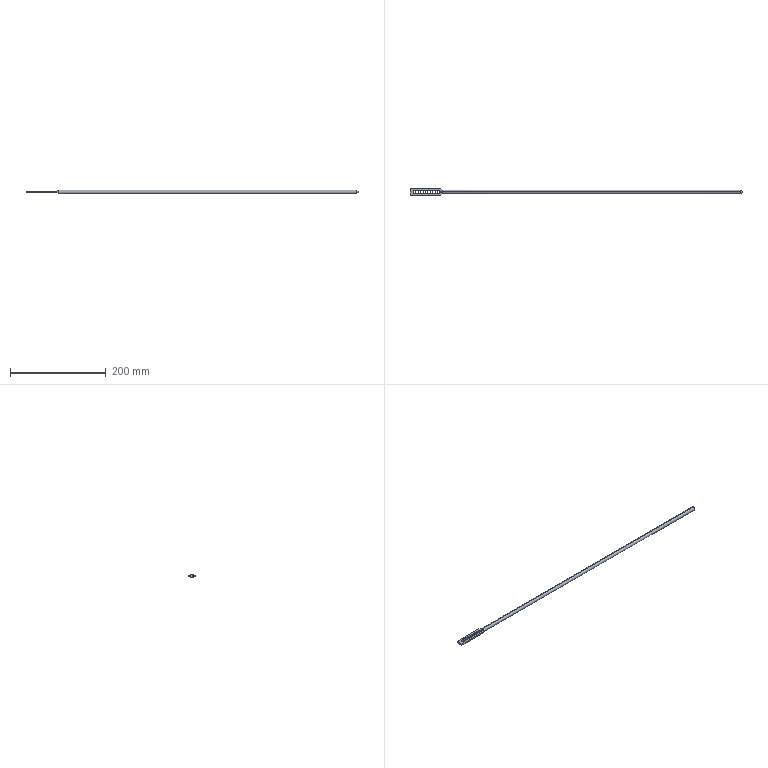Part | SolidWorks | 1 solid | 36 faces | box 695 x 14 x 8 mm | volume 33732 mm3 | cylinder 23 | plane 8 | cone 5 | commonest cylinder face diameters 6.1 x21 8 x2
STEP:
#1=CARTESIAN_POINT('',(67.,3.597,1.75));
#2=VERTEX_POINT('',#1);
#3=CARTESIAN_POINT('',(67.,0.,4.));
#4=VERTEX_POINT('',#3);
#5=CARTESIAN_POINT('',(67.,0.,0.));
#6=DIRECTION('',(1.,0.,0.));
#7=DIRECTION('',(0.,0.,-1.));
#8=AXIS2_PLACEMENT_3D('',#5,#6,#7);
#9=CIRCLE('',#8,4.);
#10=EDGE_CURVE('',#2,#4,#9,.T.);
#11=ORIENTED_EDGE('',*,*,#10,.T.);
#12=CARTESIAN_POINT('',(692.,0.,4.));
#13=VERTEX_POINT('',#12);
#14=CARTESIAN_POINT('',(695.,0.,4.));
#15=DIRECTION('',(1.,0.,0.));
#16=VECTOR('',#15,1000.);
#17=LINE('',#14,#16);
#18=EDGE_CURVE('',#4,#13,#17,.T.);
#19=ORIENTED_EDGE('',*,*,#18,.T.);
#20=CARTESIAN_POINT('',(692.,0.,-4.));
#21=VERTEX_POINT('',#20);
#22=CARTESIAN_POINT('',(692.,0.,0.));
#23=DIRECTION('',(-1.,0.,0.));
#24=DIRECTION('',(0.,0.,-1.));
#25=AXIS2_PLACEMENT_3D('',#22,#23,#24);
#26=CIRCLE('',#25,4.);
#27=EDGE_CURVE('',#13,#21,#26,.T.);
#28=ORIENTED_EDGE('',*,*,#27,.T.);
#29=CARTESIAN_POINT('',(67.,0.,-4.));
#30=VERTEX_POINT('',#29);
#31=CARTESIAN_POINT('',(695.,0.,-4.));
#32=DIRECTION('',(1.,0.,0.));
#33=VECTOR('',#32,1000.);
#34=LINE('',#31,#33);
#35=EDGE_CURVE('',#30,#21,#34,.T.);
#36=ORIENTED_EDGE('',*,*,#35,.F.);
#37=CARTESIAN_POINT('',(67.,3.597,-1.75));
#38=VERTEX_POINT('',#37);
#39=CARTESIAN_POINT('',(67.,0.,0.));
#40=DIRECTION('',(1.,0.,0.));
#41=DIRECTION('',(0.,0.,-1.));
#42=AXIS2_PLACEMENT_3D('',#39,#40,#41);
#43=CIRCLE('',#42,4.);
#44=EDGE_CURVE('',#30,#38,#43,.T.);
#45=ORIENTED_EDGE('',*,*,#44,.T.);
#46=CARTESIAN_POINT('',(67.903,3.597,-1.75));
#47=VERTEX_POINT('',#46);
#48=CARTESIAN_POINT('',(68.,3.597,-1.75));
#49=DIRECTION('',(1.,0.,0.));
#50=VECTOR('',#49,1000.);
#51=LINE('',#48,#50);
#52=EDGE_CURVE('',#38,#47,#51,.T.);
#53=ORIENTED_EDGE('',*,*,#52,.T.);
#54=CARTESIAN_POINT('',(67.903,3.597,1.75));
#55=VERTEX_POINT('',#54);
#56=CARTESIAN_POINT('',(67.903,3.597,-1.75));
#57=CARTESIAN_POINT('',(67.356,4.144,-0.6253));
#58=CARTESIAN_POINT('',(67.356,4.144,0.6253));
#59=CARTESIAN_POINT('',(67.903,3.597,1.75));
#60=(BOUNDED_CURVE()B_SPLINE_CURVE(3,(#56,#57,#58,#59),.UNSPECIFIED.,.F.,.F.)B_SPLINE_CURVE_WITH_KNOTS((4,4),(2.689,3.594),.UNSPECIFIED.)CURVE()GEOMETRIC_REPRESENTATION_ITEM()RATIONAL_B_SPLINE_CURVE((1.,0.9328,0.9328,1.))REPRESENTATION_ITEM(''));
#61=EDGE_CURVE('',#47,#55,#60,.T.);
#62=ORIENTED_EDGE('',*,*,#61,.T.);
#63=CARTESIAN_POINT('',(0.,3.597,1.75));
#64=DIRECTION('',(-1.,0.,0.));
#65=VECTOR('',#64,1000.);
#66=LINE('',#63,#65);
#67=EDGE_CURVE('',#55,#2,#66,.T.);
#68=ORIENTED_EDGE('',*,*,#67,.T.);
#69=EDGE_LOOP('',(#11,#19,#28,#36,#45,#53,#62,#68));
#70=FACE_OUTER_BOUND('',#69,.T.);
#71=CARTESIAN_POINT('',(695.,0.,0.));
#72=DIRECTION('',(1.,0.,0.));
#73=DIRECTION('',(0.,0.,-1.));
#74=AXIS2_PLACEMENT_3D('',#71,#72,#73);
#75=CYLINDRICAL_SURFACE('',#74,4.);
#76=ADVANCED_FACE('',(#70),#75,.T.);
#77=CARTESIAN_POINT('',(67.,-3.597,-1.75));
#78=VERTEX_POINT('',#77);
#79=CARTESIAN_POINT('',(65.678,0.,-1.75));
#80=VERTEX_POINT('',#79);
#81=CARTESIAN_POINT('',(67.,-3.597,-1.75));
#82=CARTESIAN_POINT('',(66.849,-3.312,-1.75));
#83=CARTESIAN_POINT('',(66.701,-3.025,-1.75));
#84=CARTESIAN_POINT('',(66.416,-2.448,-1.75));
#85=CARTESIAN_POINT('',(66.277,-2.157,-1.75));
#86=CARTESIAN_POINT('',(66.024,-1.564,-1.75));
#87=CARTESIAN_POINT('',(65.907,-1.262,-1.75));
#88=CARTESIAN_POINT('',(65.777,-0.7984,-1.75));
#89=CARTESIAN_POINT('',(65.741,-0.642,-1.75));
#90=CARTESIAN_POINT('',(65.692,-0.3236,-1.75));
#91=CARTESIAN_POINT('',(65.678,-0.1604,-1.75));
#92=CARTESIAN_POINT('',(65.678,0.,-1.75));
#93=B_SPLINE_CURVE_WITH_KNOTS('',3,(#81,#82,#83,#84,#85,#86,#87,#88,#89,#90,#91,#92),.UNSPECIFIED.,.F.,.F.,(4,2,2,2,2,4),(0.,0.0009664,0.001933,0.002899,0.003382,0.003866),.UNSPECIFIED.);
#94=EDGE_CURVE('',#78,#80,#93,.T.);
#95=ORIENTED_EDGE('',*,*,#94,.T.);
#96=CARTESIAN_POINT('',(67.,0.,-4.));
#97=DIRECTION('',(0.5065,0.,-0.8622));
#98=VECTOR('',#97,1000.);
#99=LINE('',#96,#98);
#100=EDGE_CURVE('',#80,#30,#99,.T.);
#101=ORIENTED_EDGE('',*,*,#100,.T.);
#102=CARTESIAN_POINT('',(67.,0.,0.));
#103=DIRECTION('',(1.,0.,0.));
#104=DIRECTION('',(0.,0.,-1.));
#105=AXIS2_PLACEMENT_3D('',#102,#103,#104);
#106=CIRCLE('',#105,4.);
#107=EDGE_CURVE('',#78,#30,#106,.T.);
#108=ORIENTED_EDGE('',*,*,#107,.F.);
#109=EDGE_LOOP('',(#95,#101,#108));
#110=FACE_OUTER_BOUND('',#109,.T.);
#111=CARTESIAN_POINT('',(67.,0.,0.));
#112=DIRECTION('',(1.,0.,0.));
#113=DIRECTION('',(0.,0.,-1.));
#114=AXIS2_PLACEMENT_3D('',#111,#112,#113);
#115=CONICAL_SURFACE('',#114,4.,1.04);
#116=ADVANCED_FACE('',(#110),#115,.T.);
#117=CARTESIAN_POINT('',(695.,0.,1.5));
#118=VERTEX_POINT('',#117);
#119=CARTESIAN_POINT('',(695.,0.,-1.5));
#120=VERTEX_POINT('',#119);
#121=CARTESIAN_POINT('',(695.,0.,0.));
#122=DIRECTION('',(-1.,0.,0.));
#123=DIRECTION('',(0.,0.,1.));
#124=AXIS2_PLACEMENT_3D('',#121,#122,#123);
#125=CIRCLE('',#124,1.5);
#126=EDGE_CURVE('',#118,#120,#125,.T.);
#127=ORIENTED_EDGE('',*,*,#126,.T.);
#128=CARTESIAN_POINT('',(692.,0.,-4.));
#129=DIRECTION('',(-0.7682,0.,-0.6402));
#130=VECTOR('',#129,1000.);
#131=LINE('',#128,#130);
#132=EDGE_CURVE('',#120,#21,#131,.T.);
#133=ORIENTED_EDGE('',*,*,#132,.T.);
#134=ORIENTED_EDGE('',*,*,#27,.F.);
#135=CARTESIAN_POINT('',(692.,0.,4.));
#136=DIRECTION('',(-0.7682,0.,0.6402));
#137=VECTOR('',#136,1000.);
#138=LINE('',#135,#137);
#139=EDGE_CURVE('',#118,#13,#138,.T.);
#140=ORIENTED_EDGE('',*,*,#139,.F.);
#141=EDGE_LOOP('',(#127,#133,#134,#140));
#142=FACE_OUTER_BOUND('',#141,.T.);
#143=CARTESIAN_POINT('',(692.,0.,0.));
#144=DIRECTION('',(-1.,0.,0.));
#145=DIRECTION('',(0.,0.,1.));
#146=AXIS2_PLACEMENT_3D('',#143,#144,#145);
#147=CONICAL_SURFACE('',#146,4.,0.6947);
#148=ADVANCED_FACE('',(#142),#147,.T.);
#149=CARTESIAN_POINT('',(12.5,1.747,1.75));
#150=VERTEX_POINT('',#149);
#151=CARTESIAN_POINT('',(6.95,0.,1.75));
#152=VERTEX_POINT('',#151);
#153=CARTESIAN_POINT('',(10.,0.,1.75));
#154=DIRECTION('',(0.,0.,1.));
#155=DIRECTION('',(-1.,0.,0.));
#156=AXIS2_PLACEMENT_3D('',#153,#154,#155);
#157=CIRCLE('',#156,3.05);
#158=EDGE_CURVE('',#150,#152,#157,.T.);
#159=ORIENTED_EDGE('',*,*,#158,.T.);
#160=CARTESIAN_POINT('',(6.95,0.,-1.75));
#161=VERTEX_POINT('',#160);
#162=CARTESIAN_POINT('',(6.95,0.,7.));
#163=DIRECTION('',(0.,0.,-1.));
#164=VECTOR('',#163,1000.);
#165=LINE('',#162,#164);
#166=EDGE_CURVE('',#152,#161,#165,.T.);
#167=ORIENTED_EDGE('',*,*,#166,.T.);
#168=CARTESIAN_POINT('',(12.5,1.747,-1.75));
#169=VERTEX_POINT('',#168);
#170=CARTESIAN_POINT('',(10.,0.,-1.75));
#171=DIRECTION('',(0.,0.,-1.));
#172=DIRECTION('',(-1.,0.,0.));
#173=AXIS2_PLACEMENT_3D('',#170,#171,#172);
#174=CIRCLE('',#173,3.05);
#175=EDGE_CURVE('',#161,#169,#174,.T.);
#176=ORIENTED_EDGE('',*,*,#175,.T.);
#177=CARTESIAN_POINT('',(12.5,1.747,7.));
#178=DIRECTION('',(0.,0.,1.));
#179=VECTOR('',#178,1000.);
#180=LINE('',#177,#179);
#181=EDGE_CURVE('',#169,#150,#180,.T.);
#182=ORIENTED_EDGE('',*,*,#181,.T.);
#183=EDGE_LOOP('',(#159,#167,#176,#182));
#184=FACE_OUTER_BOUND('',#183,.T.);
#185=CARTESIAN_POINT('',(10.,0.,7.));
#186=DIRECTION('',(0.,0.,-1.));
#187=DIRECTION('',(-1.,0.,0.));
#188=AXIS2_PLACEMENT_3D('',#185,#186,#187);
#189=CYLINDRICAL_SURFACE('',#188,3.05);
#190=ADVANCED_FACE('',(#184),#189,.F.);
#191=ORIENTED_EDGE('',*,*,#18,.F.);
#192=CARTESIAN_POINT('',(67.,-3.597,1.75));
#193=VERTEX_POINT('',#192);
#194=CARTESIAN_POINT('',(67.,0.,0.));
#195=DIRECTION('',(1.,0.,0.));
#196=DIRECTION('',(0.,0.,-1.));
#197=AXIS2_PLACEMENT_3D('',#194,#195,#196);
#198=CIRCLE('',#197,4.);
#199=EDGE_CURVE('',#4,#193,#198,.T.);
#200=ORIENTED_EDGE('',*,*,#199,.T.);
#201=CARTESIAN_POINT('',(67.903,-3.597,1.75));
#202=VERTEX_POINT('',#201);
#203=CARTESIAN_POINT('',(0.,-3.597,1.75));
#204=DIRECTION('',(1.,0.,0.));
#205=VECTOR('',#204,1000.);
#206=LINE('',#203,#205);
#207=EDGE_CURVE('',#193,#202,#206,.T.);
#208=ORIENTED_EDGE('',*,*,#207,.T.);
#209=CARTESIAN_POINT('',(67.903,-3.597,-1.75));
#210=VERTEX_POINT('',#209);
#211=CARTESIAN_POINT('',(67.903,-3.597,1.75));
#212=CARTESIAN_POINT('',(67.356,-4.144,0.6253));
#213=CARTESIAN_POINT('',(67.356,-4.144,-0.6253));
#214=CARTESIAN_POINT('',(67.903,-3.597,-1.75));
#215=(BOUNDED_CURVE()B_SPLINE_CURVE(3,(#211,#212,#213,#214),.UNSPECIFIED.,.F.,.F.)B_SPLINE_CURVE_WITH_KNOTS((4,4),(2.689,3.594),.UNSPECIFIED.)CURVE()GEOMETRIC_REPRESENTATION_ITEM()RATIONAL_B_SPLINE_CURVE((1.,0.9328,0.9328,1.))REPRESENTATION_ITEM(''));
#216=EDGE_CURVE('',#202,#210,#215,.T.);
#217=ORIENTED_EDGE('',*,*,#216,.T.);
#218=CARTESIAN_POINT('',(68.,-3.597,-1.75));
#219=DIRECTION('',(-1.,0.,0.));
#220=VECTOR('',#219,1000.);
#221=LINE('',#218,#220);
#222=EDGE_CURVE('',#210,#78,#221,.T.);
#223=ORIENTED_EDGE('',*,*,#222,.T.);
#224=ORIENTED_EDGE('',*,*,#107,.T.);
#225=ORIENTED_EDGE('',*,*,#35,.T.);
#226=CARTESIAN_POINT('',(692.,0.,0.));
#227=DIRECTION('',(-1.,0.,0.));
#228=DIRECTION('',(0.,0.,-1.));
#229=AXIS2_PLACEMENT_3D('',#226,#227,#228);
#230=CIRCLE('',#229,4.);
#231=EDGE_CURVE('',#21,#13,#230,.T.);
#232=ORIENTED_EDGE('',*,*,#231,.T.);
#233=EDGE_LOOP('',(#191,#200,#208,#217,#223,#224,#225,#232));
#234=FACE_OUTER_BOUND('',#233,.T.);
#235=CARTESIAN_POINT('',(695.,0.,0.));
#236=DIRECTION('',(1.,0.,0.));
#237=DIRECTION('',(0.,0.,-1.));
#238=AXIS2_PLACEMENT_3D('',#235,#236,#237);
#239=CYLINDRICAL_SURFACE('',#238,4.);
#240=ADVANCED_FACE('',(#234),#239,.T.);
#241=ORIENTED_EDGE('',*,*,#216,.F.);
#242=CARTESIAN_POINT('',(64.5,-7.,1.75));
#243=VERTEX_POINT('',#242);
#244=CARTESIAN_POINT('',(68.,-3.5,1.75));
#245=DIRECTION('',(0.7071,0.7071,0.));
#246=VECTOR('',#245,1000.);
#247=LINE('',#244,#246);
#248=EDGE_CURVE('',#243,#202,#247,.T.);
#249=ORIENTED_EDGE('',*,*,#248,.F.);
#250=CARTESIAN_POINT('',(64.5,-7.,-1.75));
#251=VERTEX_POINT('',#250);
#252=CARTESIAN_POINT('',(64.5,-7.,1.75));
#253=DIRECTION('',(0.,0.,1.));
#254=VECTOR('',#253,1000.);
#255=LINE('',#252,#254);
#256=EDGE_CURVE('',#251,#243,#255,.T.);
#257=ORIENTED_EDGE('',*,*,#256,.F.);
#258=CARTESIAN_POINT('',(68.,-3.5,-1.75));
#259=DIRECTION('',(-0.7071,-0.7071,0.));
#260=VECTOR('',#259,1000.);
#261=LINE('',#258,#260);
#262=EDGE_CURVE('',#210,#251,#261,.T.);
#263=ORIENTED_EDGE('',*,*,#262,.F.);
#264=EDGE_LOOP('',(#241,#249,#257,#263));
#265=FACE_OUTER_BOUND('',#264,.T.);
#266=CARTESIAN_POINT('',(68.,-3.5,1.75));
#267=DIRECTION('',(-0.7071,0.7071,0.));
#268=DIRECTION('',(-0.7071,-0.7071,0.));
#269=AXIS2_PLACEMENT_3D('',#266,#267,#268);
#270=PLANE('',#269);
#271=ADVANCED_FACE('',(#265),#270,.F.);
#272=ORIENTED_EDGE('',*,*,#10,.F.);
#273=CARTESIAN_POINT('',(67.,3.597,1.75));
#274=CARTESIAN_POINT('',(66.849,3.311,1.75));
#275=CARTESIAN_POINT('',(66.701,3.024,1.75));
#276=CARTESIAN_POINT('',(66.414,2.445,1.75));
#277=CARTESIAN_POINT('',(66.276,2.153,1.75));
#278=CARTESIAN_POINT('',(66.022,1.559,1.75));
#279=CARTESIAN_POINT('',(65.905,1.255,1.75));
#280=CARTESIAN_POINT('',(65.775,0.7905,1.75));
#281=CARTESIAN_POINT('',(65.74,0.6336,1.75));
#282=CARTESIAN_POINT('',(65.691,0.3142,1.75));
#283=CARTESIAN_POINT('',(65.678,0.1505,1.75));
#284=CARTESIAN_POINT('',(65.679,-0.3318,1.75));
#285=CARTESIAN_POINT('',(65.734,-0.6464,1.75));
#286=CARTESIAN_POINT('',(65.909,-1.267,1.75));
#287=CARTESIAN_POINT('',(66.026,-1.569,1.75));
#288=CARTESIAN_POINT('',(66.279,-2.16,1.75));
#289=CARTESIAN_POINT('',(66.417,-2.45,1.75));
#290=CARTESIAN_POINT('',(66.702,-3.027,1.75));
#291=CARTESIAN_POINT('',(66.85,-3.312,1.75));
#292=CARTESIAN_POINT('',(67.,-3.597,1.75));
#293=B_SPLINE_CURVE_WITH_KNOTS('',3,(#273,#274,#275,#276,#277,#278,#279,#280,#281,#282,#283,#284,#285,#286,#287,#288,#289,#290,#291,#292),.UNSPECIFIED.,.F.,.F.,(4,2,2,2,2,2,2,2,2,4),(0.,0.000969,0.001938,0.002907,0.003392,0.003876,0.004845,0.005814,0.006783,0.007752),.UNSPECIFIED.);
#294=EDGE_CURVE('',#2,#193,#293,.T.);
#295=ORIENTED_EDGE('',*,*,#294,.T.);
#296=ORIENTED_EDGE('',*,*,#199,.F.);
#297=EDGE_LOOP('',(#272,#295,#296));
#298=FACE_OUTER_BOUND('',#297,.T.);
#299=CARTESIAN_POINT('',(67.,0.,0.));
#300=DIRECTION('',(1.,0.,0.));
#301=DIRECTION('',(0.,0.,-1.));
#302=AXIS2_PLACEMENT_3D('',#299,#300,#301);
#303=CONICAL_SURFACE('',#302,4.,1.04);
#304=ADVANCED_FACE('',(#298),#303,.T.);
#305=CARTESIAN_POINT('',(64.5,7.,-1.75));
#306=VERTEX_POINT('',#305);
#307=CARTESIAN_POINT('',(64.5,7.,-1.75));
#308=DIRECTION('',(-0.7071,0.7071,0.));
#309=VECTOR('',#308,1000.);
#310=LINE('',#307,#309);
#311=EDGE_CURVE('',#47,#306,#310,.T.);
#312=ORIENTED_EDGE('',*,*,#311,.T.);
#313=CARTESIAN_POINT('',(64.5,7.,1.75));
#314=VERTEX_POINT('',#313);
#315=CARTESIAN_POINT('',(64.5,7.,0.));
#316=DIRECTION('',(0.,0.,1.));
#317=VECTOR('',#316,1000.);
#318=LINE('',#315,#317);
#319=EDGE_CURVE('',#306,#314,#318,.T.);
#320=ORIENTED_EDGE('',*,*,#319,.T.);
#321=CARTESIAN_POINT('',(64.5,7.,1.75));
#322=DIRECTION('',(0.7071,-0.7071,0.));
#323=VECTOR('',#322,1000.);
#324=LINE('',#321,#323);
#325=EDGE_CURVE('',#314,#55,#324,.T.);
#326=ORIENTED_EDGE('',*,*,#325,.T.);
#327=ORIENTED_EDGE('',*,*,#61,.F.);
#328=EDGE_LOOP('',(#312,#320,#326,#327));
#329=FACE_OUTER_BOUND('',#328,.T.);
#330=CARTESIAN_POINT('',(64.5,7.,0.));
#331=DIRECTION('',(0.7071,0.7071,0.));
#332=DIRECTION('',(-0.7071,0.7071,0.));
#333=AXIS2_PLACEMENT_3D('',#330,#331,#332);
#334=PLANE('',#333);
#335=ADVANCED_FACE('',(#329),#334,.T.);
#336=ORIENTED_EDGE('',*,*,#100,.F.);
#337=CARTESIAN_POINT('',(65.678,0.,-1.75));
#338=CARTESIAN_POINT('',(65.678,0.3225,-1.75));
#339=CARTESIAN_POINT('',(65.732,0.6381,-1.75));
#340=CARTESIAN_POINT('',(65.907,1.261,-1.75));
#341=CARTESIAN_POINT('',(66.024,1.564,-1.75));
#342=CARTESIAN_POINT('',(66.277,2.156,-1.75));
#343=CARTESIAN_POINT('',(66.415,2.447,-1.75));
#344=CARTESIAN_POINT('',(66.701,3.025,-1.75));
#345=CARTESIAN_POINT('',(66.849,3.312,-1.75));
#346=CARTESIAN_POINT('',(67.,3.597,-1.75));
#347=B_SPLINE_CURVE_WITH_KNOTS('',3,(#337,#338,#339,#340,#341,#342,#343,#344,#345,#346),.UNSPECIFIED.,.F.,.F.,(4,2,2,2,4),(0.003866,0.004837,0.005809,0.00678,0.007752),.UNSPECIFIED.);
#348=EDGE_CURVE('',#80,#38,#347,.T.);
#349=ORIENTED_EDGE('',*,*,#348,.T.);
#350=ORIENTED_EDGE('',*,*,#44,.F.);
#351=EDGE_LOOP('',(#336,#349,#350));
#352=FACE_OUTER_BOUND('',#351,.T.);
#353=CARTESIAN_POINT('',(67.,0.,0.));
#354=DIRECTION('',(1.,0.,0.));
#355=DIRECTION('',(0.,0.,-1.));
#356=AXIS2_PLACEMENT_3D('',#353,#354,#355);
#357=CONICAL_SURFACE('',#356,4.,1.04);
#358=ADVANCED_FACE('',(#352),#357,.T.);
#359=ORIENTED_EDGE('',*,*,#132,.F.);
#360=CARTESIAN_POINT('',(695.,0.,0.));
#361=DIRECTION('',(-1.,0.,0.));
#362=DIRECTION('',(0.,0.,1.));
#363=AXIS2_PLACEMENT_3D('',#360,#361,#362);
#364=CIRCLE('',#363,1.5);
#365=EDGE_CURVE('',#120,#118,#364,.T.);
#366=ORIENTED_EDGE('',*,*,#365,.T.);
#367=ORIENTED_EDGE('',*,*,#139,.T.);
#368=ORIENTED_EDGE('',*,*,#231,.F.);
#369=EDGE_LOOP('',(#359,#366,#367,#368));
#370=FACE_OUTER_BOUND('',#369,.T.);
#371=CARTESIAN_POINT('',(692.,0.,0.));
#372=DIRECTION('',(-1.,0.,0.));
#373=DIRECTION('',(0.,0.,1.));
#374=AXIS2_PLACEMENT_3D('',#371,#372,#373);
#375=CONICAL_SURFACE('',#374,4.,0.6947);
#376=ADVANCED_FACE('',(#370),#375,.T.);
#377=ORIENTED_EDGE('',*,*,#262,.T.);
#378=CARTESIAN_POINT('',(0.,-7.,-1.75));
#379=VERTEX_POINT('',#378);
#380=CARTESIAN_POINT('',(68.,-7.,-1.75));
#381=DIRECTION('',(1.,0.,0.));
#382=VECTOR('',#381,1000.);
#383=LINE('',#380,#382);
#384=EDGE_CURVE('',#379,#251,#383,.T.);
#385=ORIENTED_EDGE('',*,*,#384,.F.);
#386=CARTESIAN_POINT('',(0.,7.,-1.75));
#387=VERTEX_POINT('',#386);
#388=CARTESIAN_POINT('',(0.,7.,-1.75));
#389=DIRECTION('',(0.,-1.,0.));
#390=VECTOR('',#389,1000.);
#391=LINE('',#388,#390);
#392=EDGE_CURVE('',#387,#379,#391,.T.);
#393=ORIENTED_EDGE('',*,*,#392,.F.);
#394=CARTESIAN_POINT('',(68.,7.,-1.75));
#395=DIRECTION('',(-1.,0.,0.));
#396=VECTOR('',#395,1000.);
#397=LINE('',#394,#396);
#398=EDGE_CURVE('',#306,#387,#397,.T.);
#399=ORIENTED_EDGE('',*,*,#398,.F.);
#400=ORIENTED_EDGE('',*,*,#311,.F.);
#401=ORIENTED_EDGE('',*,*,#52,.F.);
#402=ORIENTED_EDGE('',*,*,#348,.F.);
#403=ORIENTED_EDGE('',*,*,#94,.F.);
#404=ORIENTED_EDGE('',*,*,#222,.F.);
#405=EDGE_LOOP('',(#377,#385,#393,#399,#400,#401,#402,#403,#404));
#406=FACE_OUTER_BOUND('',#405,.T.);
#407=CARTESIAN_POINT('',(22.5,-1.747,-1.75));
#408=VERTEX_POINT('',#407);
#409=CARTESIAN_POINT('',(17.5,-1.747,-1.75));
#410=VERTEX_POINT('',#409);
#411=CARTESIAN_POINT('',(20.,0.,-1.75));
#412=DIRECTION('',(0.,0.,-1.));
#413=DIRECTION('',(-1.,0.,0.));
#414=AXIS2_PLACEMENT_3D('',#411,#412,#413);
#415=CIRCLE('',#414,3.05);
#416=EDGE_CURVE('',#408,#410,#415,.T.);
#417=ORIENTED_EDGE('',*,*,#416,.F.);
#418=CARTESIAN_POINT('',(27.5,-1.747,-1.75));
#419=VERTEX_POINT('',#418);
#420=CARTESIAN_POINT('',(25.,0.,-1.75));
#421=DIRECTION('',(0.,0.,-1.));
#422=DIRECTION('',(-1.,0.,0.));
#423=AXIS2_PLACEMENT_3D('',#420,#421,#422);
#424=CIRCLE('',#423,3.05);
#425=EDGE_CURVE('',#419,#408,#424,.T.);
#426=ORIENTED_EDGE('',*,*,#425,.F.);
#427=CARTESIAN_POINT('',(32.5,-1.747,-1.75));
#428=VERTEX_POINT('',#427);
#429=CARTESIAN_POINT('',(30.,0.,-1.75));
#430=DIRECTION('',(0.,0.,-1.));
#431=DIRECTION('',(-1.,0.,0.));
#432=AXIS2_PLACEMENT_3D('',#429,#430,#431);
#433=CIRCLE('',#432,3.05);
#434=EDGE_CURVE('',#428,#419,#433,.T.);
#435=ORIENTED_EDGE('',*,*,#434,.F.);
#436=CARTESIAN_POINT('',(37.5,-1.747,-1.75));
#437=VERTEX_POINT('',#436);
#438=CARTESIAN_POINT('',(35.,0.,-1.75));
#439=DIRECTION('',(0.,0.,-1.));
#440=DIRECTION('',(-1.,0.,0.));
#441=AXIS2_PLACEMENT_3D('',#438,#439,#440);
#442=CIRCLE('',#441,3.05);
#443=EDGE_CURVE('',#437,#428,#442,.T.);
#444=ORIENTED_EDGE('',*,*,#443,.F.);
#445=CARTESIAN_POINT('',(42.5,-1.747,-1.75));
#446=VERTEX_POINT('',#445);
#447=CARTESIAN_POINT('',(40.,0.,-1.75));
#448=DIRECTION('',(0.,0.,-1.));
#449=DIRECTION('',(-1.,0.,0.));
#450=AXIS2_PLACEMENT_3D('',#447,#448,#449);
#451=CIRCLE('',#450,3.05);
#452=EDGE_CURVE('',#446,#437,#451,.T.);
#453=ORIENTED_EDGE('',*,*,#452,.F.);
#454=CARTESIAN_POINT('',(47.5,-1.747,-1.75));
#455=VERTEX_POINT('',#454);
#456=CARTESIAN_POINT('',(45.,0.,-1.75));
#457=DIRECTION('',(0.,0.,-1.));
#458=DIRECTION('',(-1.,0.,0.));
#459=AXIS2_PLACEMENT_3D('',#456,#457,#458);
#460=CIRCLE('',#459,3.05);
#461=EDGE_CURVE('',#455,#446,#460,.T.);
#462=ORIENTED_EDGE('',*,*,#461,.F.);
#463=CARTESIAN_POINT('',(52.5,-1.747,-1.75));
#464=VERTEX_POINT('',#463);
#465=CARTESIAN_POINT('',(50.,0.,-1.75));
#466=DIRECTION('',(0.,0.,-1.));
#467=DIRECTION('',(-1.,0.,0.));
#468=AXIS2_PLACEMENT_3D('',#465,#466,#467);
#469=CIRCLE('',#468,3.05);
#470=EDGE_CURVE('',#464,#455,#469,.T.);
#471=ORIENTED_EDGE('',*,*,#470,.F.);
#472=CARTESIAN_POINT('',(57.5,-1.747,-1.75));
#473=VERTEX_POINT('',#472);
#474=CARTESIAN_POINT('',(55.,0.,-1.75));
#475=DIRECTION('',(0.,0.,-1.));
#476=DIRECTION('',(-1.,0.,0.));
#477=AXIS2_PLACEMENT_3D('',#474,#475,#476);
#478=CIRCLE('',#477,3.05);
#479=EDGE_CURVE('',#473,#464,#478,.T.);
#480=ORIENTED_EDGE('',*,*,#479,.F.);
#481=CARTESIAN_POINT('',(57.5,1.747,-1.75));
#482=VERTEX_POINT('',#481);
#483=CARTESIAN_POINT('',(60.,0.,-1.75));
#484=DIRECTION('',(0.,0.,-1.));
#485=DIRECTION('',(-1.,0.,0.));
#486=AXIS2_PLACEMENT_3D('',#483,#484,#485);
#487=CIRCLE('',#486,3.05);
#488=EDGE_CURVE('',#482,#473,#487,.T.);
#489=ORIENTED_EDGE('',*,*,#488,.F.);
#490=CARTESIAN_POINT('',(52.5,1.747,-1.75));
#491=VERTEX_POINT('',#490);
#492=CARTESIAN_POINT('',(55.,0.,-1.75));
#493=DIRECTION('',(0.,0.,-1.));
#494=DIRECTION('',(-1.,0.,0.));
#495=AXIS2_PLACEMENT_3D('',#492,#493,#494);
#496=CIRCLE('',#495,3.05);
#497=EDGE_CURVE('',#491,#482,#496,.T.);
#498=ORIENTED_EDGE('',*,*,#497,.F.);
#499=CARTESIAN_POINT('',(47.5,1.747,-1.75));
#500=VERTEX_POINT('',#499);
#501=CARTESIAN_POINT('',(50.,0.,-1.75));
#502=DIRECTION('',(0.,0.,-1.));
#503=DIRECTION('',(-1.,0.,0.));
#504=AXIS2_PLACEMENT_3D('',#501,#502,#503);
#505=CIRCLE('',#504,3.05);
#506=EDGE_CURVE('',#500,#491,#505,.T.);
#507=ORIENTED_EDGE('',*,*,#506,.F.);
#508=CARTESIAN_POINT('',(42.5,1.747,-1.75));
#509=VERTEX_POINT('',#508);
#510=CARTESIAN_POINT('',(45.,0.,-1.75));
#511=DIRECTION('',(0.,0.,-1.));
#512=DIRECTION('',(-1.,0.,0.));
#513=AXIS2_PLACEMENT_3D('',#510,#511,#512);
#514=CIRCLE('',#513,3.05);
#515=EDGE_CURVE('',#509,#500,#514,.T.);
#516=ORIENTED_EDGE('',*,*,#515,.F.);
#517=CARTESIAN_POINT('',(37.5,1.747,-1.75));
#518=VERTEX_POINT('',#517);
#519=CARTESIAN_POINT('',(40.,0.,-1.75));
#520=DIRECTION('',(0.,0.,-1.));
#521=DIRECTION('',(-1.,0.,0.));
#522=AXIS2_PLACEMENT_3D('',#519,#520,#521);
#523=CIRCLE('',#522,3.05);
#524=EDGE_CURVE('',#518,#509,#523,.T.);
#525=ORIENTED_EDGE('',*,*,#524,.F.);
#526=CARTESIAN_POINT('',(32.5,1.747,-1.75));
#527=VERTEX_POINT('',#526);
#528=CARTESIAN_POINT('',(35.,0.,-1.75));
#529=DIRECTION('',(0.,0.,-1.));
#530=DIRECTION('',(-1.,0.,0.));
#531=AXIS2_PLACEMENT_3D('',#528,#529,#530);
#532=CIRCLE('',#531,3.05);
#533=EDGE_CURVE('',#527,#518,#532,.T.);
#534=ORIENTED_EDGE('',*,*,#533,.F.);
#535=CARTESIAN_POINT('',(27.5,1.747,-1.75));
#536=VERTEX_POINT('',#535);
#537=CARTESIAN_POINT('',(30.,0.,-1.75));
#538=DIRECTION('',(0.,0.,-1.));
#539=DIRECTION('',(-1.,0.,0.));
#540=AXIS2_PLACEMENT_3D('',#537,#538,#539);
#541=CIRCLE('',#540,3.05);
#542=EDGE_CURVE('',#536,#527,#541,.T.);
#543=ORIENTED_EDGE('',*,*,#542,.F.);
#544=CARTESIAN_POINT('',(22.5,1.747,-1.75));
#545=VERTEX_POINT('',#544);
#546=CARTESIAN_POINT('',(25.,0.,-1.75));
#547=DIRECTION('',(0.,0.,-1.));
#548=DIRECTION('',(-1.,0.,0.));
#549=AXIS2_PLACEMENT_3D('',#546,#547,#548);
#550=CIRCLE('',#549,3.05);
#551=EDGE_CURVE('',#545,#536,#550,.T.);
#552=ORIENTED_EDGE('',*,*,#551,.F.);
#553=CARTESIAN_POINT('',(17.5,1.747,-1.75));
#554=VERTEX_POINT('',#553);
#555=CARTESIAN_POINT('',(20.,0.,-1.75));
#556=DIRECTION('',(0.,0.,-1.));
#557=DIRECTION('',(-1.,0.,0.));
#558=AXIS2_PLACEMENT_3D('',#555,#556,#557);
#559=CIRCLE('',#558,3.05);
#560=EDGE_CURVE('',#554,#545,#559,.T.);
#561=ORIENTED_EDGE('',*,*,#560,.F.);
#562=CARTESIAN_POINT('',(15.,0.,-1.75));
#563=DIRECTION('',(0.,0.,-1.));
#564=DIRECTION('',(-1.,0.,0.));
#565=AXIS2_PLACEMENT_3D('',#562,#563,#564);
#566=CIRCLE('',#565,3.05);
#567=EDGE_CURVE('',#169,#554,#566,.T.);
#568=ORIENTED_EDGE('',*,*,#567,.F.);
#569=ORIENTED_EDGE('',*,*,#175,.F.);
#570=CARTESIAN_POINT('',(12.5,-1.747,-1.75));
#571=VERTEX_POINT('',#570);
#572=CARTESIAN_POINT('',(10.,0.,-1.75));
#573=DIRECTION('',(0.,0.,-1.));
#574=DIRECTION('',(-1.,0.,0.));
#575=AXIS2_PLACEMENT_3D('',#572,#573,#574);
#576=CIRCLE('',#575,3.05);
#577=EDGE_CURVE('',#571,#161,#576,.T.);
#578=ORIENTED_EDGE('',*,*,#577,.F.);
#579=CARTESIAN_POINT('',(15.,0.,-1.75));
#580=DIRECTION('',(0.,0.,-1.));
#581=DIRECTION('',(-1.,0.,0.));
#582=AXIS2_PLACEMENT_3D('',#579,#580,#581);
#583=CIRCLE('',#582,3.05);
#584=EDGE_CURVE('',#410,#571,#583,.T.);
#585=ORIENTED_EDGE('',*,*,#584,.F.);
#586=EDGE_LOOP('',(#417,#426,#435,#444,#453,#462,#471,#480,#489,#498,#507,#516,#525,#534,#543,#552,#561,#568,#569,#578,#585));
#587=FACE_BOUND('',#586,.T.);
#588=CARTESIAN_POINT('',(68.,7.,-1.75));
#589=DIRECTION('',(0.,0.,1.));
#590=DIRECTION('',(1.,0.,0.));
#591=AXIS2_PLACEMENT_3D('',#588,#589,#590);
#592=PLANE('',#591);
#593=ADVANCED_FACE('',(#406,#587),#592,.F.);
#594=ORIENTED_EDGE('',*,*,#325,.F.);
#595=CARTESIAN_POINT('',(0.,7.,1.75));
#596=VERTEX_POINT('',#595);
#597=CARTESIAN_POINT('',(0.,7.,1.75));
#598=DIRECTION('',(1.,0.,0.));
#599=VECTOR('',#598,1000.);
#600=LINE('',#597,#599);
#601=EDGE_CURVE('',#596,#314,#600,.T.);
#602=ORIENTED_EDGE('',*,*,#601,.F.);
#603=CARTESIAN_POINT('',(0.,-7.,1.75));
#604=VERTEX_POINT('',#603);
#605=CARTESIAN_POINT('',(0.,7.,1.75));
#606=DIRECTION('',(0.,1.,0.));
#607=VECTOR('',#606,1000.);
#608=LINE('',#605,#607);
#609=EDGE_CURVE('',#604,#596,#608,.T.);
#610=ORIENTED_EDGE('',*,*,#609,.F.);
#611=CARTESIAN_POINT('',(0.,-7.,1.75));
#612=DIRECTION('',(-1.,0.,0.));
#613=VECTOR('',#612,1000.);
#614=LINE('',#611,#613);
#615=EDGE_CURVE('',#243,#604,#614,.T.);
#616=ORIENTED_EDGE('',*,*,#615,.F.);
#617=ORIENTED_EDGE('',*,*,#248,.T.);
#618=ORIENTED_EDGE('',*,*,#207,.F.);
#619=ORIENTED_EDGE('',*,*,#294,.F.);
#620=ORIENTED_EDGE('',*,*,#67,.F.);
#621=EDGE_LOOP('',(#594,#602,#610,#616,#617,#618,#619,#620));
#622=FACE_OUTER_BOUND('',#621,.T.);
#623=CARTESIAN_POINT('',(22.5,1.747,1.75));
#624=VERTEX_POINT('',#623);
#625=CARTESIAN_POINT('',(17.5,1.747,1.75));
#626=VERTEX_POINT('',#625);
#627=CARTESIAN_POINT('',(20.,0.,1.75));
#628=DIRECTION('',(0.,0.,1.));
#629=DIRECTION('',(-1.,0.,0.));
#630=AXIS2_PLACEMENT_3D('',#627,#628,#629);
#631=CIRCLE('',#630,3.05);
#632=EDGE_CURVE('',#624,#626,#631,.T.);
#633=ORIENTED_EDGE('',*,*,#632,.F.);
#634=CARTESIAN_POINT('',(27.5,1.747,1.75));
#635=VERTEX_POINT('',#634);
#636=CARTESIAN_POINT('',(25.,0.,1.75));
#637=DIRECTION('',(0.,0.,1.));
#638=DIRECTION('',(-1.,0.,0.));
#639=AXIS2_PLACEMENT_3D('',#636,#637,#638);
#640=CIRCLE('',#639,3.05);
#641=EDGE_CURVE('',#635,#624,#640,.T.);
#642=ORIENTED_EDGE('',*,*,#641,.F.);
#643=CARTESIAN_POINT('',(32.5,1.747,1.75));
#644=VERTEX_POINT('',#643);
#645=CARTESIAN_POINT('',(30.,0.,1.75));
#646=DIRECTION('',(0.,0.,1.));
#647=DIRECTION('',(-1.,0.,0.));
#648=AXIS2_PLACEMENT_3D('',#645,#646,#647);
#649=CIRCLE('',#648,3.05);
#650=EDGE_CURVE('',#644,#635,#649,.T.);
#651=ORIENTED_EDGE('',*,*,#650,.F.);
#652=CARTESIAN_POINT('',(37.5,1.747,1.75));
#653=VERTEX_POINT('',#652);
#654=CARTESIAN_POINT('',(35.,0.,1.75));
#655=DIRECTION('',(0.,0.,1.));
#656=DIRECTION('',(-1.,0.,0.));
#657=AXIS2_PLACEMENT_3D('',#654,#655,#656);
#658=CIRCLE('',#657,3.05);
#659=EDGE_CURVE('',#653,#644,#658,.T.);
#660=ORIENTED_EDGE('',*,*,#659,.F.);
#661=CARTESIAN_POINT('',(42.5,1.747,1.75));
#662=VERTEX_POINT('',#661);
#663=CARTESIAN_POINT('',(40.,0.,1.75));
#664=DIRECTION('',(0.,0.,1.));
#665=DIRECTION('',(-1.,0.,0.));
#666=AXIS2_PLACEMENT_3D('',#663,#664,#665);
#667=CIRCLE('',#666,3.05);
#668=EDGE_CURVE('',#662,#653,#667,.T.);
#669=ORIENTED_EDGE('',*,*,#668,.F.);
#670=CARTESIAN_POINT('',(47.5,1.747,1.75));
#671=VERTEX_POINT('',#670);
#672=CARTESIAN_POINT('',(45.,0.,1.75));
#673=DIRECTION('',(0.,0.,1.));
#674=DIRECTION('',(-1.,0.,0.));
#675=AXIS2_PLACEMENT_3D('',#672,#673,#674);
#676=CIRCLE('',#675,3.05);
#677=EDGE_CURVE('',#671,#662,#676,.T.);
#678=ORIENTED_EDGE('',*,*,#677,.F.);
#679=CARTESIAN_POINT('',(52.5,1.747,1.75));
#680=VERTEX_POINT('',#679);
#681=CARTESIAN_POINT('',(50.,0.,1.75));
#682=DIRECTION('',(0.,0.,1.));
#683=DIRECTION('',(-1.,0.,0.));
#684=AXIS2_PLACEMENT_3D('',#681,#682,#683);
#685=CIRCLE('',#684,3.05);
#686=EDGE_CURVE('',#680,#671,#685,.T.);
#687=ORIENTED_EDGE('',*,*,#686,.F.);
#688=CARTESIAN_POINT('',(57.5,1.747,1.75));
#689=VERTEX_POINT('',#688);
#690=CARTESIAN_POINT('',(55.,0.,1.75));
#691=DIRECTION('',(0.,0.,1.));
#692=DIRECTION('',(-1.,0.,0.));
#693=AXIS2_PLACEMENT_3D('',#690,#691,#692);
#694=CIRCLE('',#693,3.05);
#695=EDGE_CURVE('',#689,#680,#694,.T.);
#696=ORIENTED_EDGE('',*,*,#695,.F.);
#697=CARTESIAN_POINT('',(57.5,-1.747,1.75));
#698=VERTEX_POINT('',#697);
#699=CARTESIAN_POINT('',(60.,0.,1.75));
#700=DIRECTION('',(0.,0.,1.));
#701=DIRECTION('',(-1.,0.,0.));
#702=AXIS2_PLACEMENT_3D('',#699,#700,#701);
#703=CIRCLE('',#702,3.05);
#704=EDGE_CURVE('',#698,#689,#703,.T.);
#705=ORIENTED_EDGE('',*,*,#704,.F.);
#706=CARTESIAN_POINT('',(52.5,-1.747,1.75));
#707=VERTEX_POINT('',#706);
#708=CARTESIAN_POINT('',(55.,0.,1.75));
#709=DIRECTION('',(0.,0.,1.));
#710=DIRECTION('',(-1.,0.,0.));
#711=AXIS2_PLACEMENT_3D('',#708,#709,#710);
#712=CIRCLE('',#711,3.05);
#713=EDGE_CURVE('',#707,#698,#712,.T.);
#714=ORIENTED_EDGE('',*,*,#713,.F.);
#715=CARTESIAN_POINT('',(47.5,-1.747,1.75));
#716=VERTEX_POINT('',#715);
#717=CARTESIAN_POINT('',(50.,0.,1.75));
#718=DIRECTION('',(0.,0.,1.));
#719=DIRECTION('',(-1.,0.,0.));
#720=AXIS2_PLACEMENT_3D('',#717,#718,#719);
#721=CIRCLE('',#720,3.05);
#722=EDGE_CURVE('',#716,#707,#721,.T.);
#723=ORIENTED_EDGE('',*,*,#722,.F.);
#724=CARTESIAN_POINT('',(42.5,-1.747,1.75));
#725=VERTEX_POINT('',#724);
#726=CARTESIAN_POINT('',(45.,0.,1.75));
#727=DIRECTION('',(0.,0.,1.));
#728=DIRECTION('',(-1.,0.,0.));
#729=AXIS2_PLACEMENT_3D('',#726,#727,#728);
#730=CIRCLE('',#729,3.05);
#731=EDGE_CURVE('',#725,#716,#730,.T.);
#732=ORIENTED_EDGE('',*,*,#731,.F.);
#733=CARTESIAN_POINT('',(37.5,-1.747,1.75));
#734=VERTEX_POINT('',#733);
#735=CARTESIAN_POINT('',(40.,0.,1.75));
#736=DIRECTION('',(0.,0.,1.));
#737=DIRECTION('',(-1.,0.,0.));
#738=AXIS2_PLACEMENT_3D('',#735,#736,#737);
#739=CIRCLE('',#738,3.05);
#740=EDGE_CURVE('',#734,#725,#739,.T.);
#741=ORIENTED_EDGE('',*,*,#740,.F.);
#742=CARTESIAN_POINT('',(32.5,-1.747,1.75));
#743=VERTEX_POINT('',#742);
#744=CARTESIAN_POINT('',(35.,0.,1.75));
#745=DIRECTION('',(0.,0.,1.));
#746=DIRECTION('',(-1.,0.,0.));
#747=AXIS2_PLACEMENT_3D('',#744,#745,#746);
#748=CIRCLE('',#747,3.05);
#749=EDGE_CURVE('',#743,#734,#748,.T.);
#750=ORIENTED_EDGE('',*,*,#749,.F.);
#751=CARTESIAN_POINT('',(27.5,-1.747,1.75));
#752=VERTEX_POINT('',#751);
#753=CARTESIAN_POINT('',(30.,0.,1.75));
#754=DIRECTION('',(0.,0.,1.));
#755=DIRECTION('',(-1.,0.,0.));
#756=AXIS2_PLACEMENT_3D('',#753,#754,#755);
#757=CIRCLE('',#756,3.05);
#758=EDGE_CURVE('',#752,#743,#757,.T.);
#759=ORIENTED_EDGE('',*,*,#758,.F.);
#760=CARTESIAN_POINT('',(22.5,-1.747,1.75));
#761=VERTEX_POINT('',#760);
#762=CARTESIAN_POINT('',(25.,0.,1.75));
#763=DIRECTION('',(0.,0.,1.));
#764=DIRECTION('',(-1.,0.,0.));
#765=AXIS2_PLACEMENT_3D('',#762,#763,#764);
#766=CIRCLE('',#765,3.05);
#767=EDGE_CURVE('',#761,#752,#766,.T.);
#768=ORIENTED_EDGE('',*,*,#767,.F.);
#769=CARTESIAN_POINT('',(17.5,-1.747,1.75));
#770=VERTEX_POINT('',#769);
#771=CARTESIAN_POINT('',(20.,0.,1.75));
#772=DIRECTION('',(0.,0.,1.));
#773=DIRECTION('',(-1.,0.,0.));
#774=AXIS2_PLACEMENT_3D('',#771,#772,#773);
#775=CIRCLE('',#774,3.05);
#776=EDGE_CURVE('',#770,#761,#775,.T.);
#777=ORIENTED_EDGE('',*,*,#776,.F.);
#778=CARTESIAN_POINT('',(12.5,-1.747,1.75));
#779=VERTEX_POINT('',#778);
#780=CARTESIAN_POINT('',(15.,0.,1.75));
#781=DIRECTION('',(0.,0.,1.));
#782=DIRECTION('',(-1.,0.,0.));
#783=AXIS2_PLACEMENT_3D('',#780,#781,#782);
#784=CIRCLE('',#783,3.05);
#785=EDGE_CURVE('',#779,#770,#784,.T.);
#786=ORIENTED_EDGE('',*,*,#785,.F.);
#787=CARTESIAN_POINT('',(10.,0.,1.75));
#788=DIRECTION('',(0.,0.,1.));
#789=DIRECTION('',(-1.,0.,0.));
#790=AXIS2_PLACEMENT_3D('',#787,#788,#789);
#791=CIRCLE('',#790,3.05);
#792=EDGE_CURVE('',#152,#779,#791,.T.);
#793=ORIENTED_EDGE('',*,*,#792,.F.);
#794=ORIENTED_EDGE('',*,*,#158,.F.);
#795=CARTESIAN_POINT('',(15.,0.,1.75));
#796=DIRECTION('',(0.,0.,1.));
#797=DIRECTION('',(-1.,0.,0.));
#798=AXIS2_PLACEMENT_3D('',#795,#796,#797);
#799=CIRCLE('',#798,3.05);
#800=EDGE_CURVE('',#626,#150,#799,.T.);
#801=ORIENTED_EDGE('',*,*,#800,.F.);
#802=EDGE_LOOP('',(#633,#642,#651,#660,#669,#678,#687,#696,#705,#714,#723,#732,#741,#750,#759,#768,#777,#786,#793,#794,#801));
#803=FACE_BOUND('',#802,.T.);
#804=CARTESIAN_POINT('',(0.,7.,1.75));
#805=DIRECTION('',(0.,0.,-1.));
#806=DIRECTION('',(-1.,0.,0.));
#807=AXIS2_PLACEMENT_3D('',#804,#805,#806);
#808=PLANE('',#807);
#809=ADVANCED_FACE('',(#622,#803),#808,.F.);
#810=ORIENTED_EDGE('',*,*,#256,.T.);
#811=ORIENTED_EDGE('',*,*,#615,.T.);
#812=CARTESIAN_POINT('',(0.,-7.,0.));
#813=DIRECTION('',(0.,0.,1.));
#814=VECTOR('',#813,1000.);
#815=LINE('',#812,#814);
#816=EDGE_CURVE('',#379,#604,#815,.T.);
#817=ORIENTED_EDGE('',*,*,#816,.F.);
#818=ORIENTED_EDGE('',*,*,#384,.T.);
#819=EDGE_LOOP('',(#810,#811,#817,#818));
#820=FACE_OUTER_BOUND('',#819,.T.);
#821=CARTESIAN_POINT('',(0.,-7.,0.));
#822=DIRECTION('',(0.,1.,0.));
#823=DIRECTION('',(0.,0.,1.));
#824=AXIS2_PLACEMENT_3D('',#821,#822,#823);
#825=PLANE('',#824);
#826=ADVANCED_FACE('',(#820),#825,.F.);
#827=ORIENTED_EDGE('',*,*,#398,.T.);
#828=CARTESIAN_POINT('',(0.,7.,0.));
#829=DIRECTION('',(0.,0.,1.));
#830=VECTOR('',#829,1000.);
#831=LINE('',#828,#830);
#832=EDGE_CURVE('',#387,#596,#831,.T.);
#833=ORIENTED_EDGE('',*,*,#832,.T.);
#834=ORIENTED_EDGE('',*,*,#601,.T.);
#835=ORIENTED_EDGE('',*,*,#319,.F.);
#836=EDGE_LOOP('',(#827,#833,#834,#835));
#837=FACE_OUTER_BOUND('',#836,.T.);
#838=CARTESIAN_POINT('',(0.,7.,0.));
#839=DIRECTION('',(0.,1.,0.));
#840=DIRECTION('',(0.,0.,1.));
#841=AXIS2_PLACEMENT_3D('',#838,#839,#840);
#842=PLANE('',#841);
#843=ADVANCED_FACE('',(#837),#842,.T.);
#844=ORIENTED_EDGE('',*,*,#126,.F.);
#845=ORIENTED_EDGE('',*,*,#365,.F.);
#846=EDGE_LOOP('',(#844,#845));
#847=FACE_OUTER_BOUND('',#846,.T.);
#848=CARTESIAN_POINT('',(695.,0.,-1.5));
#849=DIRECTION('',(-1.,0.,0.));
#850=DIRECTION('',(0.,0.,1.));
#851=AXIS2_PLACEMENT_3D('',#848,#849,#850);
#852=PLANE('',#851);
#853=ADVANCED_FACE('',(#847),#852,.F.);
#854=ORIENTED_EDGE('',*,*,#609,.T.);
#855=ORIENTED_EDGE('',*,*,#832,.F.);
#856=ORIENTED_EDGE('',*,*,#392,.T.);
#857=ORIENTED_EDGE('',*,*,#816,.T.);
#858=EDGE_LOOP('',(#854,#855,#856,#857));
#859=FACE_OUTER_BOUND('',#858,.T.);
#860=CARTESIAN_POINT('',(0.,7.,-1.75));
#861=DIRECTION('',(1.,0.,0.));
#862=DIRECTION('',(0.,0.,-1.));
#863=AXIS2_PLACEMENT_3D('',#860,#861,#862);
#864=PLANE('',#863);
#865=ADVANCED_FACE('',(#859),#864,.F.);
#866=CARTESIAN_POINT('',(12.5,-1.747,7.));
#867=DIRECTION('',(0.,0.,-1.));
#868=VECTOR('',#867,1000.);
#869=LINE('',#866,#868);
#870=EDGE_CURVE('',#779,#571,#869,.T.);
#871=ORIENTED_EDGE('',*,*,#870,.F.);
#872=ORIENTED_EDGE('',*,*,#785,.T.);
#873=CARTESIAN_POINT('',(17.5,-1.747,7.));
#874=DIRECTION('',(0.,0.,1.));
#875=VECTOR('',#874,1000.);
#876=LINE('',#873,#875);
#877=EDGE_CURVE('',#410,#770,#876,.T.);
#878=ORIENTED_EDGE('',*,*,#877,.F.);
#879=ORIENTED_EDGE('',*,*,#584,.T.);
#880=EDGE_LOOP('',(#871,#872,#878,#879));
#881=FACE_OUTER_BOUND('',#880,.T.);
#882=CARTESIAN_POINT('',(15.,0.,7.));
#883=DIRECTION('',(0.,0.,-1.));
#884=DIRECTION('',(-1.,0.,0.));
#885=AXIS2_PLACEMENT_3D('',#882,#883,#884);
#886=CYLINDRICAL_SURFACE('',#885,3.05);
#887=ADVANCED_FACE('',(#881),#886,.F.);
#888=ORIENTED_EDGE('',*,*,#877,.T.);
#889=ORIENTED_EDGE('',*,*,#776,.T.);
#890=CARTESIAN_POINT('',(22.5,-1.747,7.));
#891=DIRECTION('',(0.,0.,1.));
#892=VECTOR('',#891,1000.);
#893=LINE('',#890,#892);
#894=EDGE_CURVE('',#408,#761,#893,.T.);
#895=ORIENTED_EDGE('',*,*,#894,.F.);
#896=ORIENTED_EDGE('',*,*,#416,.T.);
#897=EDGE_LOOP('',(#888,#889,#895,#896));
#898=FACE_OUTER_BOUND('',#897,.T.);
#899=CARTESIAN_POINT('',(20.,0.,7.));
#900=DIRECTION('',(0.,0.,-1.));
#901=DIRECTION('',(-1.,0.,0.));
#902=AXIS2_PLACEMENT_3D('',#899,#900,#901);
#903=CYLINDRICAL_SURFACE('',#902,3.05);
#904=ADVANCED_FACE('',(#898),#903,.F.);
#905=ORIENTED_EDGE('',*,*,#894,.T.);
#906=ORIENTED_EDGE('',*,*,#767,.T.);
#907=CARTESIAN_POINT('',(27.5,-1.747,7.));
#908=DIRECTION('',(0.,0.,1.));
#909=VECTOR('',#908,1000.);
#910=LINE('',#907,#909);
#911=EDGE_CURVE('',#419,#752,#910,.T.);
#912=ORIENTED_EDGE('',*,*,#911,.F.);
#913=ORIENTED_EDGE('',*,*,#425,.T.);
#914=EDGE_LOOP('',(#905,#906,#912,#913));
#915=FACE_OUTER_BOUND('',#914,.T.);
#916=CARTESIAN_POINT('',(25.,0.,7.));
#917=DIRECTION('',(0.,0.,-1.));
#918=DIRECTION('',(-1.,0.,0.));
#919=AXIS2_PLACEMENT_3D('',#916,#917,#918);
#920=CYLINDRICAL_SURFACE('',#919,3.05);
#921=ADVANCED_FACE('',(#915),#920,.F.);
#922=ORIENTED_EDGE('',*,*,#911,.T.);
#923=ORIENTED_EDGE('',*,*,#758,.T.);
#924=CARTESIAN_POINT('',(32.5,-1.747,7.));
#925=DIRECTION('',(0.,0.,1.));
#926=VECTOR('',#925,1000.);
#927=LINE('',#924,#926);
#928=EDGE_CURVE('',#428,#743,#927,.T.);
#929=ORIENTED_EDGE('',*,*,#928,.F.);
#930=ORIENTED_EDGE('',*,*,#434,.T.);
#931=EDGE_LOOP('',(#922,#923,#929,#930));
#932=FACE_OUTER_BOUND('',#931,.T.);
#933=CARTESIAN_POINT('',(30.,0.,7.));
#934=DIRECTION('',(0.,0.,-1.));
#935=DIRECTION('',(-1.,0.,0.));
#936=AXIS2_PLACEMENT_3D('',#933,#934,#935);
#937=CYLINDRICAL_SURFACE('',#936,3.05);
#938=ADVANCED_FACE('',(#932),#937,.F.);
#939=ORIENTED_EDGE('',*,*,#928,.T.);
#940=ORIENTED_EDGE('',*,*,#749,.T.);
#941=CARTESIAN_POINT('',(37.5,-1.747,7.));
#942=DIRECTION('',(0.,0.,1.));
#943=VECTOR('',#942,1000.);
#944=LINE('',#941,#943);
#945=EDGE_CURVE('',#437,#734,#944,.T.);
#946=ORIENTED_EDGE('',*,*,#945,.F.);
#947=ORIENTED_EDGE('',*,*,#443,.T.);
#948=EDGE_LOOP('',(#939,#940,#946,#947));
#949=FACE_OUTER_BOUND('',#948,.T.);
#950=CARTESIAN_POINT('',(35.,0.,7.));
#951=DIRECTION('',(0.,0.,-1.));
#952=DIRECTION('',(-1.,0.,0.));
#953=AXIS2_PLACEMENT_3D('',#950,#951,#952);
#954=CYLINDRICAL_SURFACE('',#953,3.05);
#955=ADVANCED_FACE('',(#949),#954,.F.);
#956=ORIENTED_EDGE('',*,*,#945,.T.);
#957=ORIENTED_EDGE('',*,*,#740,.T.);
#958=CARTESIAN_POINT('',(42.5,-1.747,7.));
#959=DIRECTION('',(0.,0.,1.));
#960=VECTOR('',#959,1000.);
#961=LINE('',#958,#960);
#962=EDGE_CURVE('',#446,#725,#961,.T.);
#963=ORIENTED_EDGE('',*,*,#962,.F.);
#964=ORIENTED_EDGE('',*,*,#452,.T.);
#965=EDGE_LOOP('',(#956,#957,#963,#964));
#966=FACE_OUTER_BOUND('',#965,.T.);
#967=CARTESIAN_POINT('',(40.,0.,7.));
#968=DIRECTION('',(0.,0.,-1.));
#969=DIRECTION('',(-1.,0.,0.));
#970=AXIS2_PLACEMENT_3D('',#967,#968,#969);
#971=CYLINDRICAL_SURFACE('',#970,3.05);
#972=ADVANCED_FACE('',(#966),#971,.F.);
#973=ORIENTED_EDGE('',*,*,#962,.T.);
#974=ORIENTED_EDGE('',*,*,#731,.T.);
#975=CARTESIAN_POINT('',(47.5,-1.747,7.));
#976=DIRECTION('',(0.,0.,1.));
#977=VECTOR('',#976,1000.);
#978=LINE('',#975,#977);
#979=EDGE_CURVE('',#455,#716,#978,.T.);
#980=ORIENTED_EDGE('',*,*,#979,.F.);
#981=ORIENTED_EDGE('',*,*,#461,.T.);
#982=EDGE_LOOP('',(#973,#974,#980,#981));
#983=FACE_OUTER_BOUND('',#982,.T.);
#984=CARTESIAN_POINT('',(45.,0.,7.));
#985=DIRECTION('',(0.,0.,-1.));
#986=DIRECTION('',(-1.,0.,0.));
#987=AXIS2_PLACEMENT_3D('',#984,#985,#986);
#988=CYLINDRICAL_SURFACE('',#987,3.05);
#989=ADVANCED_FACE('',(#983),#988,.F.);
#990=ORIENTED_EDGE('',*,*,#979,.T.);
#991=ORIENTED_EDGE('',*,*,#722,.T.);
#992=CARTESIAN_POINT('',(52.5,-1.747,7.));
#993=DIRECTION('',(0.,0.,1.));
#994=VECTOR('',#993,1000.);
#995=LINE('',#992,#994);
#996=EDGE_CURVE('',#464,#707,#995,.T.);
#997=ORIENTED_EDGE('',*,*,#996,.F.);
#998=ORIENTED_EDGE('',*,*,#470,.T.);
#999=EDGE_LOOP('',(#990,#991,#997,#998));
#1000=FACE_OUTER_BOUND('',#999,.T.);
#1001=CARTESIAN_POINT('',(50.,0.,7.));
#1002=DIRECTION('',(0.,0.,-1.));
#1003=DIRECTION('',(-1.,0.,0.));
#1004=AXIS2_PLACEMENT_3D('',#1001,#1002,#1003);
#1005=CYLINDRICAL_SURFACE('',#1004,3.05);
#1006=ADVANCED_FACE('',(#1000),#1005,.F.);
#1007=ORIENTED_EDGE('',*,*,#996,.T.);
#1008=ORIENTED_EDGE('',*,*,#713,.T.);
#1009=CARTESIAN_POINT('',(57.5,-1.747,7.));
#1010=DIRECTION('',(0.,0.,1.));
#1011=VECTOR('',#1010,1000.);
#1012=LINE('',#1009,#1011);
#1013=EDGE_CURVE('',#473,#698,#1012,.T.);
#1014=ORIENTED_EDGE('',*,*,#1013,.F.);
#1015=ORIENTED_EDGE('',*,*,#479,.T.);
#1016=EDGE_LOOP('',(#1007,#1008,#1014,#1015));
#1017=FACE_OUTER_BOUND('',#1016,.T.);
#1018=CARTESIAN_POINT('',(55.,0.,7.));
#1019=DIRECTION('',(0.,0.,-1.));
#1020=DIRECTION('',(-1.,0.,0.));
#1021=AXIS2_PLACEMENT_3D('',#1018,#1019,#1020);
#1022=CYLINDRICAL_SURFACE('',#1021,3.05);
#1023=ADVANCED_FACE('',(#1017),#1022,.F.);
#1024=ORIENTED_EDGE('',*,*,#1013,.T.);
#1025=ORIENTED_EDGE('',*,*,#704,.T.);
#1026=CARTESIAN_POINT('',(57.5,1.747,7.));
#1027=DIRECTION('',(0.,0.,1.));
#1028=VECTOR('',#1027,1000.);
#1029=LINE('',#1026,#1028);
#1030=EDGE_CURVE('',#482,#689,#1029,.T.);
#1031=ORIENTED_EDGE('',*,*,#1030,.F.);
#1032=ORIENTED_EDGE('',*,*,#488,.T.);
#1033=EDGE_LOOP('',(#1024,#1025,#1031,#1032));
#1034=FACE_OUTER_BOUND('',#1033,.T.);
#1035=CARTESIAN_POINT('',(60.,0.,7.));
#1036=DIRECTION('',(0.,0.,-1.));
#1037=DIRECTION('',(-1.,0.,0.));
#1038=AXIS2_PLACEMENT_3D('',#1035,#1036,#1037);
#1039=CYLINDRICAL_SURFACE('',#1038,3.05);
#1040=ADVANCED_FACE('',(#1034),#1039,.F.);
#1041=ORIENTED_EDGE('',*,*,#1030,.T.);
#1042=ORIENTED_EDGE('',*,*,#695,.T.);
#1043=CARTESIAN_POINT('',(52.5,1.747,7.));
#1044=DIRECTION('',(0.,0.,1.));
#1045=VECTOR('',#1044,1000.);
#1046=LINE('',#1043,#1045);
#1047=EDGE_CURVE('',#491,#680,#1046,.T.);
#1048=ORIENTED_EDGE('',*,*,#1047,.F.);
#1049=ORIENTED_EDGE('',*,*,#497,.T.);
#1050=EDGE_LOOP('',(#1041,#1042,#1048,#1049));
#1051=FACE_OUTER_BOUND('',#1050,.T.);
#1052=CARTESIAN_POINT('',(55.,0.,7.));
#1053=DIRECTION('',(0.,0.,-1.));
#1054=DIRECTION('',(-1.,0.,0.));
#1055=AXIS2_PLACEMENT_3D('',#1052,#1053,#1054);
#1056=CYLINDRICAL_SURFACE('',#1055,3.05);
#1057=ADVANCED_FACE('',(#1051),#1056,.F.);
#1058=ORIENTED_EDGE('',*,*,#1047,.T.);
#1059=ORIENTED_EDGE('',*,*,#686,.T.);
#1060=CARTESIAN_POINT('',(47.5,1.747,7.));
#1061=DIRECTION('',(0.,0.,1.));
#1062=VECTOR('',#1061,1000.);
#1063=LINE('',#1060,#1062);
#1064=EDGE_CURVE('',#500,#671,#1063,.T.);
#1065=ORIENTED_EDGE('',*,*,#1064,.F.);
#1066=ORIENTED_EDGE('',*,*,#506,.T.);
#1067=EDGE_LOOP('',(#1058,#1059,#1065,#1066));
#1068=FACE_OUTER_BOUND('',#1067,.T.);
#1069=CARTESIAN_POINT('',(50.,0.,7.));
#1070=DIRECTION('',(0.,0.,-1.));
#1071=DIRECTION('',(-1.,0.,0.));
#1072=AXIS2_PLACEMENT_3D('',#1069,#1070,#1071);
#1073=CYLINDRICAL_SURFACE('',#1072,3.05);
#1074=ADVANCED_FACE('',(#1068),#1073,.F.);
#1075=ORIENTED_EDGE('',*,*,#1064,.T.);
#1076=ORIENTED_EDGE('',*,*,#677,.T.);
#1077=CARTESIAN_POINT('',(42.5,1.747,7.));
#1078=DIRECTION('',(0.,0.,1.));
#1079=VECTOR('',#1078,1000.);
#1080=LINE('',#1077,#1079);
#1081=EDGE_CURVE('',#509,#662,#1080,.T.);
#1082=ORIENTED_EDGE('',*,*,#1081,.F.);
#1083=ORIENTED_EDGE('',*,*,#515,.T.);
#1084=EDGE_LOOP('',(#1075,#1076,#1082,#1083));
#1085=FACE_OUTER_BOUND('',#1084,.T.);
#1086=CARTESIAN_POINT('',(45.,0.,7.));
#1087=DIRECTION('',(0.,0.,-1.));
#1088=DIRECTION('',(-1.,0.,0.));
#1089=AXIS2_PLACEMENT_3D('',#1086,#1087,#1088);
#1090=CYLINDRICAL_SURFACE('',#1089,3.05);
#1091=ADVANCED_FACE('',(#1085),#1090,.F.);
#1092=ORIENTED_EDGE('',*,*,#1081,.T.);
#1093=ORIENTED_EDGE('',*,*,#668,.T.);
#1094=CARTESIAN_POINT('',(37.5,1.747,7.));
#1095=DIRECTION('',(0.,0.,1.));
#1096=VECTOR('',#1095,1000.);
#1097=LINE('',#1094,#1096);
#1098=EDGE_CURVE('',#518,#653,#1097,.T.);
#1099=ORIENTED_EDGE('',*,*,#1098,.F.);
#1100=ORIENTED_EDGE('',*,*,#524,.T.);
#1101=EDGE_LOOP('',(#1092,#1093,#1099,#1100));
#1102=FACE_OUTER_BOUND('',#1101,.T.);
#1103=CARTESIAN_POINT('',(40.,0.,7.));
#1104=DIRECTION('',(0.,0.,-1.));
#1105=DIRECTION('',(-1.,0.,0.));
#1106=AXIS2_PLACEMENT_3D('',#1103,#1104,#1105);
#1107=CYLINDRICAL_SURFACE('',#1106,3.05);
#1108=ADVANCED_FACE('',(#1102),#1107,.F.);
#1109=ORIENTED_EDGE('',*,*,#1098,.T.);
#1110=ORIENTED_EDGE('',*,*,#659,.T.);
#1111=CARTESIAN_POINT('',(32.5,1.747,7.));
#1112=DIRECTION('',(0.,0.,1.));
#1113=VECTOR('',#1112,1000.);
#1114=LINE('',#1111,#1113);
#1115=EDGE_CURVE('',#527,#644,#1114,.T.);
#1116=ORIENTED_EDGE('',*,*,#1115,.F.);
#1117=ORIENTED_EDGE('',*,*,#533,.T.);
#1118=EDGE_LOOP('',(#1109,#1110,#1116,#1117));
#1119=FACE_OUTER_BOUND('',#1118,.T.);
#1120=CARTESIAN_POINT('',(35.,0.,7.));
#1121=DIRECTION('',(0.,0.,-1.));
#1122=DIRECTION('',(-1.,0.,0.));
#1123=AXIS2_PLACEMENT_3D('',#1120,#1121,#1122);
#1124=CYLINDRICAL_SURFACE('',#1123,3.05);
#1125=ADVANCED_FACE('',(#1119),#1124,.F.);
#1126=ORIENTED_EDGE('',*,*,#1115,.T.);
#1127=ORIENTED_EDGE('',*,*,#650,.T.);
#1128=CARTESIAN_POINT('',(27.5,1.747,7.));
#1129=DIRECTION('',(0.,0.,1.));
#1130=VECTOR('',#1129,1000.);
#1131=LINE('',#1128,#1130);
#1132=EDGE_CURVE('',#536,#635,#1131,.T.);
#1133=ORIENTED_EDGE('',*,*,#1132,.F.);
#1134=ORIENTED_EDGE('',*,*,#542,.T.);
#1135=EDGE_LOOP('',(#1126,#1127,#1133,#1134));
#1136=FACE_OUTER_BOUND('',#1135,.T.);
#1137=CARTESIAN_POINT('',(30.,0.,7.));
#1138=DIRECTION('',(0.,0.,-1.));
#1139=DIRECTION('',(-1.,0.,0.));
#1140=AXIS2_PLACEMENT_3D('',#1137,#1138,#1139);
#1141=CYLINDRICAL_SURFACE('',#1140,3.05);
#1142=ADVANCED_FACE('',(#1136),#1141,.F.);
#1143=ORIENTED_EDGE('',*,*,#1132,.T.);
#1144=ORIENTED_EDGE('',*,*,#641,.T.);
#1145=CARTESIAN_POINT('',(22.5,1.747,7.));
#1146=DIRECTION('',(0.,0.,1.));
#1147=VECTOR('',#1146,1000.);
#1148=LINE('',#1145,#1147);
#1149=EDGE_CURVE('',#545,#624,#1148,.T.);
#1150=ORIENTED_EDGE('',*,*,#1149,.F.);
#1151=ORIENTED_EDGE('',*,*,#551,.T.);
#1152=EDGE_LOOP('',(#1143,#1144,#1150,#1151));
#1153=FACE_OUTER_BOUND('',#1152,.T.);
#1154=CARTESIAN_POINT('',(25.,0.,7.));
#1155=DIRECTION('',(0.,0.,-1.));
#1156=DIRECTION('',(-1.,0.,0.));
#1157=AXIS2_PLACEMENT_3D('',#1154,#1155,#1156);
#1158=CYLINDRICAL_SURFACE('',#1157,3.05);
#1159=ADVANCED_FACE('',(#1153),#1158,.F.);
#1160=ORIENTED_EDGE('',*,*,#1149,.T.);
#1161=ORIENTED_EDGE('',*,*,#632,.T.);
#1162=CARTESIAN_POINT('',(17.5,1.747,7.));
#1163=DIRECTION('',(0.,0.,1.));
#1164=VECTOR('',#1163,1000.);
#1165=LINE('',#1162,#1164);
#1166=EDGE_CURVE('',#554,#626,#1165,.T.);
#1167=ORIENTED_EDGE('',*,*,#1166,.F.);
#1168=ORIENTED_EDGE('',*,*,#560,.T.);
#1169=EDGE_LOOP('',(#1160,#1161,#1167,#1168));
#1170=FACE_OUTER_BOUND('',#1169,.T.);
#1171=CARTESIAN_POINT('',(20.,0.,7.));
#1172=DIRECTION('',(0.,0.,-1.));
#1173=DIRECTION('',(-1.,0.,0.));
#1174=AXIS2_PLACEMENT_3D('',#1171,#1172,#1173);
#1175=CYLINDRICAL_SURFACE('',#1174,3.05);
#1176=ADVANCED_FACE('',(#1170),#1175,.F.);
#1177=ORIENTED_EDGE('',*,*,#1166,.T.);
#1178=ORIENTED_EDGE('',*,*,#800,.T.);
#1179=ORIENTED_EDGE('',*,*,#181,.F.);
#1180=ORIENTED_EDGE('',*,*,#567,.T.);
#1181=EDGE_LOOP('',(#1177,#1178,#1179,#1180));
#1182=FACE_OUTER_BOUND('',#1181,.T.);
#1183=CARTESIAN_POINT('',(15.,0.,7.));
#1184=DIRECTION('',(0.,0.,-1.));
#1185=DIRECTION('',(-1.,0.,0.));
#1186=AXIS2_PLACEMENT_3D('',#1183,#1184,#1185);
#1187=CYLINDRICAL_SURFACE('',#1186,3.05);
#1188=ADVANCED_FACE('',(#1182),#1187,.F.);
#1189=ORIENTED_EDGE('',*,*,#166,.F.);
#1190=ORIENTED_EDGE('',*,*,#792,.T.);
#1191=ORIENTED_EDGE('',*,*,#870,.T.);
#1192=ORIENTED_EDGE('',*,*,#577,.T.);
#1193=EDGE_LOOP('',(#1189,#1190,#1191,#1192));
#1194=FACE_OUTER_BOUND('',#1193,.T.);
#1195=CARTESIAN_POINT('',(10.,0.,7.));
#1196=DIRECTION('',(0.,0.,-1.));
#1197=DIRECTION('',(-1.,0.,0.));
#1198=AXIS2_PLACEMENT_3D('',#1195,#1196,#1197);
#1199=CYLINDRICAL_SURFACE('',#1198,3.05);
#1200=ADVANCED_FACE('',(#1194),#1199,.F.);
#1201=CLOSED_SHELL('',(#76,#116,#148,#190,#240,#271,#304,#335,#358,#376,#593,#809,#826,#843,#853,#865,#887,#904,#921,#938,#955,#972,#989,#1006,#1023,#1040,#1057,#1074,#1091,#1108,#1125,#1142,#1159,#1176,#1188,#1200));
#1202=MANIFOLD_SOLID_BREP('',#1201);
#1203=CARTESIAN_POINT('',(0.,0.,0.));
#1204=DIRECTION('',(0.,0.,1.));
#1205=DIRECTION('',(1.,0.,0.));
#1206=AXIS2_PLACEMENT_3D('',#1203,#1204,#1205);
#1207=(LENGTH_UNIT()NAMED_UNIT(*)SI_UNIT(.MILLI.,.METRE.));
#1208=UNCERTAINTY_MEASURE_WITH_UNIT(LENGTH_MEASURE(0.00001),#1207,'','');
#1209=(NAMED_UNIT(*)PLANE_ANGLE_UNIT()SI_UNIT($,.RADIAN.));
#1210=(NAMED_UNIT(*)SI_UNIT($,.STERADIAN.)SOLID_ANGLE_UNIT());
#1211=(GEOMETRIC_REPRESENTATION_CONTEXT(3)GLOBAL_UNCERTAINTY_ASSIGNED_CONTEXT((#1208))GLOBAL_UNIT_ASSIGNED_CONTEXT((#1207,#1209,#1210))REPRESENTATION_CONTEXT('',''));
#1212=ADVANCED_BREP_SHAPE_REPRESENTATION('',(#1202,#1206),#1211);